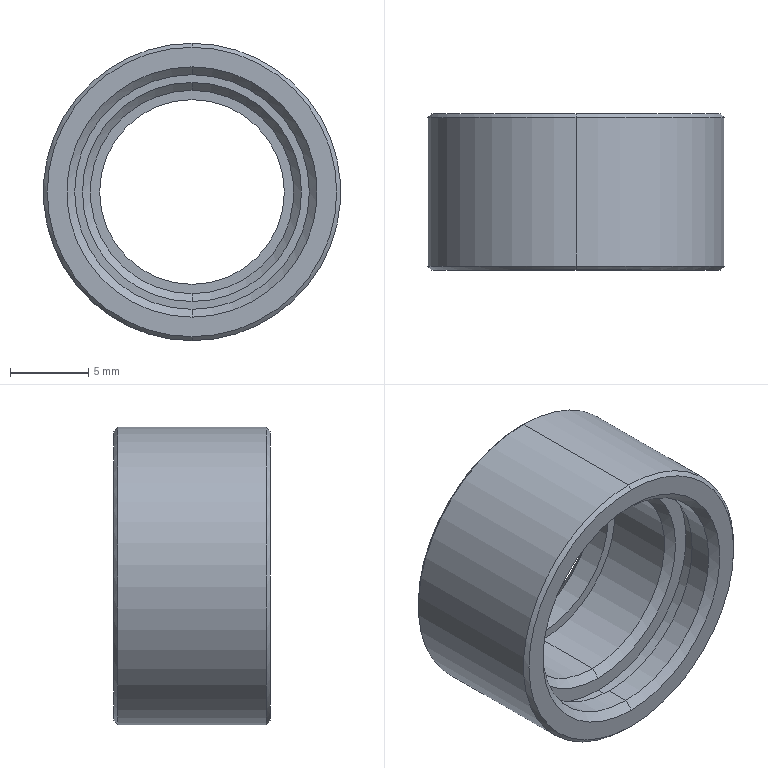Part | NX | features BREP 1 | 1 solid | 25 faces | box 19 x 10 x 19 mm | volume 1381 mm3 | cone 10 | cylinder 10 | plane 5 | commonest cylinder face diameters 11.8 x2 13 x2 15 x2 15.9 x2 19 x2
STEP:
#1=CARTESIAN_POINT('',(0.,0.25,-9.5));
#2=VERTEX_POINT('',#1);
#3=CARTESIAN_POINT('',(0.,0.,-9.25));
#4=VERTEX_POINT('',#3);
#5=CARTESIAN_POINT('',(0.,0.,-9.25));
#6=DIRECTION('',(0.,0.7071,-0.7071));
#7=VECTOR('',#6,1000.);
#8=LINE('',#5,#7);
#9=EDGE_CURVE('',#2,#4,#8,.F.);
#10=ORIENTED_EDGE('',*,*,#9,.T.);
#11=CARTESIAN_POINT('',(0.,0.,9.25));
#12=VERTEX_POINT('',#11);
#13=CARTESIAN_POINT('',(0.,0.,0.));
#14=DIRECTION('',(0.,-1.,0.));
#15=DIRECTION('',(0.,0.,1.));
#16=AXIS2_PLACEMENT_3D('',#13,#14,#15);
#17=CIRCLE('',#16,9.25);
#18=EDGE_CURVE('',#12,#4,#17,.T.);
#19=ORIENTED_EDGE('',*,*,#18,.F.);
#20=CARTESIAN_POINT('',(0.,0.25,9.5));
#21=VERTEX_POINT('',#20);
#22=CARTESIAN_POINT('',(0.,0.,9.25));
#23=DIRECTION('',(0.,0.7071,0.7071));
#24=VECTOR('',#23,1000.);
#25=LINE('',#22,#24);
#26=EDGE_CURVE('',#21,#12,#25,.F.);
#27=ORIENTED_EDGE('',*,*,#26,.F.);
#28=CARTESIAN_POINT('',(0.,0.25,0.));
#29=DIRECTION('',(0.,1.,0.));
#30=DIRECTION('',(0.,0.,1.));
#31=AXIS2_PLACEMENT_3D('',#28,#29,#30);
#32=CIRCLE('',#31,9.5);
#33=EDGE_CURVE('',#2,#21,#32,.T.);
#34=ORIENTED_EDGE('',*,*,#33,.F.);
#35=EDGE_LOOP('',(#10,#19,#27,#34));
#36=FACE_BOUND('',#35,.T.);
#37=CARTESIAN_POINT('',(0.,0.,0.));
#38=DIRECTION('',(0.,1.,0.));
#39=DIRECTION('',(0.,0.,1.));
#40=AXIS2_PLACEMENT_3D('',#37,#38,#39);
#41=CONICAL_SURFACE('',#40,9.25,0.7854);
#42=ADVANCED_FACE('',(#36),#41,.T.);
#43=CARTESIAN_POINT('',(0.,10.,9.25));
#44=VERTEX_POINT('',#43);
#45=CARTESIAN_POINT('',(0.,9.75,9.5));
#46=VERTEX_POINT('',#45);
#47=CARTESIAN_POINT('',(0.,9.75,9.5));
#48=DIRECTION('',(0.,-0.7071,0.7071));
#49=VECTOR('',#48,1000.);
#50=LINE('',#47,#49);
#51=EDGE_CURVE('',#44,#46,#50,.T.);
#52=ORIENTED_EDGE('',*,*,#51,.F.);
#53=CARTESIAN_POINT('',(0.,10.,-9.25));
#54=VERTEX_POINT('',#53);
#55=CARTESIAN_POINT('',(0.,10.,0.));
#56=DIRECTION('',(0.,1.,0.));
#57=DIRECTION('',(0.,0.,-1.));
#58=AXIS2_PLACEMENT_3D('',#55,#56,#57);
#59=CIRCLE('',#58,9.25);
#60=EDGE_CURVE('',#54,#44,#59,.T.);
#61=ORIENTED_EDGE('',*,*,#60,.F.);
#62=CARTESIAN_POINT('',(0.,9.75,-9.5));
#63=VERTEX_POINT('',#62);
#64=CARTESIAN_POINT('',(0.,9.75,-9.5));
#65=DIRECTION('',(0.,-0.7071,-0.7071));
#66=VECTOR('',#65,1000.);
#67=LINE('',#64,#66);
#68=EDGE_CURVE('',#54,#63,#67,.T.);
#69=ORIENTED_EDGE('',*,*,#68,.T.);
#70=CARTESIAN_POINT('',(0.,9.75,0.));
#71=DIRECTION('',(0.,-1.,0.));
#72=DIRECTION('',(0.,0.,-1.));
#73=AXIS2_PLACEMENT_3D('',#70,#71,#72);
#74=CIRCLE('',#73,9.5);
#75=EDGE_CURVE('',#46,#63,#74,.T.);
#76=ORIENTED_EDGE('',*,*,#75,.F.);
#77=EDGE_LOOP('',(#52,#61,#69,#76));
#78=FACE_BOUND('',#77,.T.);
#79=CARTESIAN_POINT('',(0.,9.75,0.));
#80=DIRECTION('',(0.,-1.,0.));
#81=DIRECTION('',(0.,0.,-1.));
#82=AXIS2_PLACEMENT_3D('',#79,#80,#81);
#83=CONICAL_SURFACE('',#82,9.5,0.7854);
#84=ADVANCED_FACE('',(#78),#83,.T.);
#85=CARTESIAN_POINT('',(0.,10.,-6.4));
#86=VERTEX_POINT('',#85);
#87=CARTESIAN_POINT('',(0.,9.5,-5.9));
#88=VERTEX_POINT('',#87);
#89=CARTESIAN_POINT('',(0.,10.,-6.4));
#90=DIRECTION('',(0.,0.7071,-0.7071));
#91=VECTOR('',#90,1000.);
#92=LINE('',#89,#91);
#93=EDGE_CURVE('',#86,#88,#92,.F.);
#94=ORIENTED_EDGE('',*,*,#93,.T.);
#95=CARTESIAN_POINT('',(0.,9.5,5.9));
#96=VERTEX_POINT('',#95);
#97=CARTESIAN_POINT('',(0.,9.5,0.));
#98=DIRECTION('',(0.,1.,0.));
#99=DIRECTION('',(0.,0.,-1.));
#100=AXIS2_PLACEMENT_3D('',#97,#98,#99);
#101=CIRCLE('',#100,5.9);
#102=EDGE_CURVE('',#96,#88,#101,.T.);
#103=ORIENTED_EDGE('',*,*,#102,.F.);
#104=CARTESIAN_POINT('',(0.,10.,6.4));
#105=VERTEX_POINT('',#104);
#106=CARTESIAN_POINT('',(0.,10.,6.4));
#107=DIRECTION('',(0.,0.7071,0.7071));
#108=VECTOR('',#107,1000.);
#109=LINE('',#106,#108);
#110=EDGE_CURVE('',#105,#96,#109,.F.);
#111=ORIENTED_EDGE('',*,*,#110,.F.);
#112=CARTESIAN_POINT('',(0.,10.,0.));
#113=DIRECTION('',(0.,-1.,0.));
#114=DIRECTION('',(0.,0.,-1.));
#115=AXIS2_PLACEMENT_3D('',#112,#113,#114);
#116=CIRCLE('',#115,6.4);
#117=EDGE_CURVE('',#86,#105,#116,.T.);
#118=ORIENTED_EDGE('',*,*,#117,.F.);
#119=EDGE_LOOP('',(#94,#103,#111,#118));
#120=FACE_BOUND('',#119,.T.);
#121=CARTESIAN_POINT('',(0.,10.,0.));
#122=DIRECTION('',(0.,1.,0.));
#123=DIRECTION('',(0.,0.,1.));
#124=AXIS2_PLACEMENT_3D('',#121,#122,#123);
#125=CONICAL_SURFACE('',#124,6.4,0.7854);
#126=ADVANCED_FACE('',(#120),#125,.F.);
#127=CARTESIAN_POINT('',(0.,3.5,6.5));
#128=VERTEX_POINT('',#127);
#129=CARTESIAN_POINT('',(0.,3.,7.));
#130=VERTEX_POINT('',#129);
#131=CARTESIAN_POINT('',(0.,3.5,6.5));
#132=DIRECTION('',(0.,-0.7071,0.7071));
#133=VECTOR('',#132,1000.);
#134=LINE('',#131,#133);
#135=EDGE_CURVE('',#128,#130,#134,.T.);
#136=ORIENTED_EDGE('',*,*,#135,.F.);
#137=CARTESIAN_POINT('',(0.,3.5,-6.5));
#138=VERTEX_POINT('',#137);
#139=CARTESIAN_POINT('',(0.,3.5,0.));
#140=DIRECTION('',(0.,-1.,0.));
#141=DIRECTION('',(0.,0.,1.));
#142=AXIS2_PLACEMENT_3D('',#139,#140,#141);
#143=CIRCLE('',#142,6.5);
#144=EDGE_CURVE('',#138,#128,#143,.T.);
#145=ORIENTED_EDGE('',*,*,#144,.F.);
#146=CARTESIAN_POINT('',(0.,3.,-7.));
#147=VERTEX_POINT('',#146);
#148=CARTESIAN_POINT('',(0.,3.5,-6.5));
#149=DIRECTION('',(0.,-0.7071,-0.7071));
#150=VECTOR('',#149,1000.);
#151=LINE('',#148,#150);
#152=EDGE_CURVE('',#138,#147,#151,.T.);
#153=ORIENTED_EDGE('',*,*,#152,.T.);
#154=CARTESIAN_POINT('',(0.,3.,0.));
#155=DIRECTION('',(0.,1.,0.));
#156=DIRECTION('',(0.,0.,1.));
#157=AXIS2_PLACEMENT_3D('',#154,#155,#156);
#158=CIRCLE('',#157,7.);
#159=EDGE_CURVE('',#130,#147,#158,.T.);
#160=ORIENTED_EDGE('',*,*,#159,.F.);
#161=EDGE_LOOP('',(#136,#145,#153,#160));
#162=FACE_BOUND('',#161,.T.);
#163=CARTESIAN_POINT('',(0.,3.5,0.));
#164=DIRECTION('',(0.,-1.,0.));
#165=DIRECTION('',(0.,0.,-1.));
#166=AXIS2_PLACEMENT_3D('',#163,#164,#165);
#167=CONICAL_SURFACE('',#166,6.5,0.7854);
#168=ADVANCED_FACE('',(#162),#167,.F.);
#169=CARTESIAN_POINT('',(0.,0.5,7.5));
#170=VERTEX_POINT('',#169);
#171=CARTESIAN_POINT('',(0.,0.,8.));
#172=VERTEX_POINT('',#171);
#173=CARTESIAN_POINT('',(0.,0.5,7.5));
#174=DIRECTION('',(0.,-0.7071,0.7071));
#175=VECTOR('',#174,1000.);
#176=LINE('',#173,#175);
#177=EDGE_CURVE('',#170,#172,#176,.T.);
#178=ORIENTED_EDGE('',*,*,#177,.F.);
#179=CARTESIAN_POINT('',(0.,0.5,-7.5));
#180=VERTEX_POINT('',#179);
#181=CARTESIAN_POINT('',(0.,0.5,0.));
#182=DIRECTION('',(0.,-1.,0.));
#183=DIRECTION('',(0.,0.,1.));
#184=AXIS2_PLACEMENT_3D('',#181,#182,#183);
#185=CIRCLE('',#184,7.5);
#186=EDGE_CURVE('',#180,#170,#185,.T.);
#187=ORIENTED_EDGE('',*,*,#186,.F.);
#188=CARTESIAN_POINT('',(0.,0.,-8.));
#189=VERTEX_POINT('',#188);
#190=CARTESIAN_POINT('',(0.,0.5,-7.5));
#191=DIRECTION('',(0.,-0.7071,-0.7071));
#192=VECTOR('',#191,1000.);
#193=LINE('',#190,#192);
#194=EDGE_CURVE('',#180,#189,#193,.T.);
#195=ORIENTED_EDGE('',*,*,#194,.T.);
#196=CARTESIAN_POINT('',(0.,0.,0.));
#197=DIRECTION('',(0.,1.,0.));
#198=DIRECTION('',(0.,0.,1.));
#199=AXIS2_PLACEMENT_3D('',#196,#197,#198);
#200=CIRCLE('',#199,8.);
#201=EDGE_CURVE('',#172,#189,#200,.T.);
#202=ORIENTED_EDGE('',*,*,#201,.F.);
#203=EDGE_LOOP('',(#178,#187,#195,#202));
#204=FACE_BOUND('',#203,.T.);
#205=CARTESIAN_POINT('',(0.,0.5,0.));
#206=DIRECTION('',(0.,-1.,0.));
#207=DIRECTION('',(0.,0.,-1.));
#208=AXIS2_PLACEMENT_3D('',#205,#206,#207);
#209=CONICAL_SURFACE('',#208,7.5,0.7854);
#210=ADVANCED_FACE('',(#204),#209,.F.);
#211=CARTESIAN_POINT('',(0.,2.,7.5));
#212=VERTEX_POINT('',#211);
#213=CARTESIAN_POINT('',(0.,0.,7.5));
#214=DIRECTION('',(0.,-1.,0.));
#215=VECTOR('',#214,1000.);
#216=LINE('',#213,#215);
#217=EDGE_CURVE('',#212,#170,#216,.T.);
#218=ORIENTED_EDGE('',*,*,#217,.F.);
#219=CARTESIAN_POINT('',(0.,2.,-7.5));
#220=VERTEX_POINT('',#219);
#221=CARTESIAN_POINT('',(0.,2.,0.));
#222=DIRECTION('',(0.,-1.,0.));
#223=DIRECTION('',(0.,0.,-1.));
#224=AXIS2_PLACEMENT_3D('',#221,#222,#223);
#225=CIRCLE('',#224,7.5);
#226=EDGE_CURVE('',#220,#212,#225,.T.);
#227=ORIENTED_EDGE('',*,*,#226,.F.);
#228=CARTESIAN_POINT('',(0.,0.,-7.5));
#229=DIRECTION('',(0.,-1.,0.));
#230=VECTOR('',#229,1000.);
#231=LINE('',#228,#230);
#232=EDGE_CURVE('',#220,#180,#231,.T.);
#233=ORIENTED_EDGE('',*,*,#232,.T.);
#234=ORIENTED_EDGE('',*,*,#186,.T.);
#235=EDGE_LOOP('',(#218,#227,#233,#234));
#236=FACE_BOUND('',#235,.T.);
#237=CARTESIAN_POINT('',(0.,0.,0.));
#238=DIRECTION('',(0.,-1.,0.));
#239=DIRECTION('',(0.,0.,-1.));
#240=AXIS2_PLACEMENT_3D('',#237,#238,#239);
#241=CYLINDRICAL_SURFACE('',#240,7.5);
#242=ADVANCED_FACE('',(#236),#241,.F.);
#243=ORIENTED_EDGE('',*,*,#226,.T.);
#244=CARTESIAN_POINT('',(0.,2.,0.));
#245=DIRECTION('',(0.,-1.,0.));
#246=DIRECTION('',(0.,0.,-1.));
#247=AXIS2_PLACEMENT_3D('',#244,#245,#246);
#248=CIRCLE('',#247,7.5);
#249=EDGE_CURVE('',#212,#220,#248,.T.);
#250=ORIENTED_EDGE('',*,*,#249,.T.);
#251=EDGE_LOOP('',(#243,#250));
#252=FACE_BOUND('',#251,.T.);
#253=CARTESIAN_POINT('',(0.,2.,-7.95));
#254=VERTEX_POINT('',#253);
#255=CARTESIAN_POINT('',(0.,2.,7.95));
#256=VERTEX_POINT('',#255);
#257=CARTESIAN_POINT('',(0.,2.,0.));
#258=DIRECTION('',(0.,-1.,0.));
#259=DIRECTION('',(0.,0.,-1.));
#260=AXIS2_PLACEMENT_3D('',#257,#258,#259);
#261=CIRCLE('',#260,7.95);
#262=EDGE_CURVE('',#254,#256,#261,.T.);
#263=ORIENTED_EDGE('',*,*,#262,.F.);
#264=CARTESIAN_POINT('',(0.,2.,0.));
#265=DIRECTION('',(0.,-1.,0.));
#266=DIRECTION('',(0.,0.,-1.));
#267=AXIS2_PLACEMENT_3D('',#264,#265,#266);
#268=CIRCLE('',#267,7.95);
#269=EDGE_CURVE('',#256,#254,#268,.T.);
#270=ORIENTED_EDGE('',*,*,#269,.F.);
#271=EDGE_LOOP('',(#263,#270));
#272=FACE_BOUND('',#271,.T.);
#273=CARTESIAN_POINT('',(-7.95,2.,0.));
#274=DIRECTION('',(0.,-1.,0.));
#275=DIRECTION('',(0.,0.,-1.));
#276=AXIS2_PLACEMENT_3D('',#273,#274,#275);
#277=PLANE('',#276);
#278=ADVANCED_FACE('',(#252,#272),#277,.F.);
#279=CARTESIAN_POINT('',(0.,3.,7.95));
#280=VERTEX_POINT('',#279);
#281=CARTESIAN_POINT('',(0.,0.,7.95));
#282=DIRECTION('',(0.,-1.,0.));
#283=VECTOR('',#282,1000.);
#284=LINE('',#281,#283);
#285=EDGE_CURVE('',#280,#256,#284,.T.);
#286=ORIENTED_EDGE('',*,*,#285,.F.);
#287=CARTESIAN_POINT('',(0.,3.,-7.95));
#288=VERTEX_POINT('',#287);
#289=CARTESIAN_POINT('',(0.,3.,0.));
#290=DIRECTION('',(0.,-1.,0.));
#291=DIRECTION('',(0.,0.,-1.));
#292=AXIS2_PLACEMENT_3D('',#289,#290,#291);
#293=CIRCLE('',#292,7.95);
#294=EDGE_CURVE('',#288,#280,#293,.T.);
#295=ORIENTED_EDGE('',*,*,#294,.F.);
#296=CARTESIAN_POINT('',(0.,0.,-7.95));
#297=DIRECTION('',(0.,-1.,0.));
#298=VECTOR('',#297,1000.);
#299=LINE('',#296,#298);
#300=EDGE_CURVE('',#288,#254,#299,.T.);
#301=ORIENTED_EDGE('',*,*,#300,.T.);
#302=ORIENTED_EDGE('',*,*,#262,.T.);
#303=EDGE_LOOP('',(#286,#295,#301,#302));
#304=FACE_BOUND('',#303,.T.);
#305=CARTESIAN_POINT('',(0.,0.,0.));
#306=DIRECTION('',(0.,-1.,0.));
#307=DIRECTION('',(0.,0.,-1.));
#308=AXIS2_PLACEMENT_3D('',#305,#306,#307);
#309=CYLINDRICAL_SURFACE('',#308,7.95);
#310=ADVANCED_FACE('',(#304),#309,.F.);
#311=ORIENTED_EDGE('',*,*,#294,.T.);
#312=CARTESIAN_POINT('',(0.,3.,0.));
#313=DIRECTION('',(0.,-1.,0.));
#314=DIRECTION('',(0.,0.,-1.));
#315=AXIS2_PLACEMENT_3D('',#312,#313,#314);
#316=CIRCLE('',#315,7.95);
#317=EDGE_CURVE('',#280,#288,#316,.T.);
#318=ORIENTED_EDGE('',*,*,#317,.T.);
#319=EDGE_LOOP('',(#311,#318));
#320=FACE_BOUND('',#319,.T.);
#321=CARTESIAN_POINT('',(0.,3.,0.));
#322=DIRECTION('',(0.,1.,0.));
#323=DIRECTION('',(0.,0.,1.));
#324=AXIS2_PLACEMENT_3D('',#321,#322,#323);
#325=CIRCLE('',#324,7.);
#326=EDGE_CURVE('',#147,#130,#325,.T.);
#327=ORIENTED_EDGE('',*,*,#326,.T.);
#328=ORIENTED_EDGE('',*,*,#159,.T.);
#329=EDGE_LOOP('',(#327,#328));
#330=FACE_BOUND('',#329,.T.);
#331=CARTESIAN_POINT('',(-6.5,3.,0.));
#332=DIRECTION('',(0.,1.,0.));
#333=DIRECTION('',(0.,0.,1.));
#334=AXIS2_PLACEMENT_3D('',#331,#332,#333);
#335=PLANE('',#334);
#336=ADVANCED_FACE('',(#320,#330),#335,.F.);
#337=CARTESIAN_POINT('',(0.,8.,6.5));
#338=VERTEX_POINT('',#337);
#339=CARTESIAN_POINT('',(0.,0.,6.5));
#340=DIRECTION('',(0.,-1.,0.));
#341=VECTOR('',#340,1000.);
#342=LINE('',#339,#341);
#343=EDGE_CURVE('',#338,#128,#342,.T.);
#344=ORIENTED_EDGE('',*,*,#343,.F.);
#345=CARTESIAN_POINT('',(0.,8.,-6.5));
#346=VERTEX_POINT('',#345);
#347=CARTESIAN_POINT('',(0.,8.,0.));
#348=DIRECTION('',(0.,-1.,0.));
#349=DIRECTION('',(0.,0.,-1.));
#350=AXIS2_PLACEMENT_3D('',#347,#348,#349);
#351=CIRCLE('',#350,6.5);
#352=EDGE_CURVE('',#346,#338,#351,.T.);
#353=ORIENTED_EDGE('',*,*,#352,.F.);
#354=CARTESIAN_POINT('',(0.,0.,-6.5));
#355=DIRECTION('',(0.,-1.,0.));
#356=VECTOR('',#355,1000.);
#357=LINE('',#354,#356);
#358=EDGE_CURVE('',#346,#138,#357,.T.);
#359=ORIENTED_EDGE('',*,*,#358,.T.);
#360=ORIENTED_EDGE('',*,*,#144,.T.);
#361=EDGE_LOOP('',(#344,#353,#359,#360));
#362=FACE_BOUND('',#361,.T.);
#363=CARTESIAN_POINT('',(0.,0.,0.));
#364=DIRECTION('',(0.,-1.,0.));
#365=DIRECTION('',(0.,0.,-1.));
#366=AXIS2_PLACEMENT_3D('',#363,#364,#365);
#367=CYLINDRICAL_SURFACE('',#366,6.5);
#368=ADVANCED_FACE('',(#362),#367,.F.);
#369=ORIENTED_EDGE('',*,*,#352,.T.);
#370=CARTESIAN_POINT('',(0.,8.,0.));
#371=DIRECTION('',(0.,-1.,0.));
#372=DIRECTION('',(0.,0.,-1.));
#373=AXIS2_PLACEMENT_3D('',#370,#371,#372);
#374=CIRCLE('',#373,6.5);
#375=EDGE_CURVE('',#338,#346,#374,.T.);
#376=ORIENTED_EDGE('',*,*,#375,.T.);
#377=EDGE_LOOP('',(#369,#376));
#378=FACE_BOUND('',#377,.T.);
#379=CARTESIAN_POINT('',(0.,8.,-5.9));
#380=VERTEX_POINT('',#379);
#381=CARTESIAN_POINT('',(0.,8.,5.9));
#382=VERTEX_POINT('',#381);
#383=CARTESIAN_POINT('',(0.,8.,0.));
#384=DIRECTION('',(0.,-1.,0.));
#385=DIRECTION('',(0.,0.,-1.));
#386=AXIS2_PLACEMENT_3D('',#383,#384,#385);
#387=CIRCLE('',#386,5.9);
#388=EDGE_CURVE('',#380,#382,#387,.T.);
#389=ORIENTED_EDGE('',*,*,#388,.F.);
#390=CARTESIAN_POINT('',(0.,8.,0.));
#391=DIRECTION('',(0.,-1.,0.));
#392=DIRECTION('',(0.,0.,-1.));
#393=AXIS2_PLACEMENT_3D('',#390,#391,#392);
#394=CIRCLE('',#393,5.9);
#395=EDGE_CURVE('',#382,#380,#394,.T.);
#396=ORIENTED_EDGE('',*,*,#395,.F.);
#397=EDGE_LOOP('',(#389,#396));
#398=FACE_BOUND('',#397,.T.);
#399=CARTESIAN_POINT('',(-5.9,8.,0.));
#400=DIRECTION('',(0.,1.,0.));
#401=DIRECTION('',(0.,0.,1.));
#402=AXIS2_PLACEMENT_3D('',#399,#400,#401);
#403=PLANE('',#402);
#404=ADVANCED_FACE('',(#378,#398),#403,.F.);
#405=CARTESIAN_POINT('',(0.,0.,5.9));
#406=DIRECTION('',(0.,-1.,0.));
#407=VECTOR('',#406,1000.);
#408=LINE('',#405,#407);
#409=EDGE_CURVE('',#96,#382,#408,.T.);
#410=ORIENTED_EDGE('',*,*,#409,.F.);
#411=ORIENTED_EDGE('',*,*,#102,.T.);
#412=CARTESIAN_POINT('',(0.,0.,-5.9));
#413=DIRECTION('',(0.,-1.,0.));
#414=VECTOR('',#413,1000.);
#415=LINE('',#412,#414);
#416=EDGE_CURVE('',#88,#380,#415,.T.);
#417=ORIENTED_EDGE('',*,*,#416,.T.);
#418=ORIENTED_EDGE('',*,*,#388,.T.);
#419=EDGE_LOOP('',(#410,#411,#417,#418));
#420=FACE_BOUND('',#419,.T.);
#421=CARTESIAN_POINT('',(0.,0.,0.));
#422=DIRECTION('',(0.,-1.,0.));
#423=DIRECTION('',(0.,0.,-1.));
#424=AXIS2_PLACEMENT_3D('',#421,#422,#423);
#425=CYLINDRICAL_SURFACE('',#424,5.9);
#426=ADVANCED_FACE('',(#420),#425,.F.);
#427=CARTESIAN_POINT('',(0.,10.,0.));
#428=DIRECTION('',(0.,-1.,0.));
#429=DIRECTION('',(0.,0.,-1.));
#430=AXIS2_PLACEMENT_3D('',#427,#428,#429);
#431=CIRCLE('',#430,6.4);
#432=EDGE_CURVE('',#105,#86,#431,.T.);
#433=ORIENTED_EDGE('',*,*,#432,.T.);
#434=ORIENTED_EDGE('',*,*,#117,.T.);
#435=EDGE_LOOP('',(#433,#434));
#436=FACE_BOUND('',#435,.T.);
#437=ORIENTED_EDGE('',*,*,#60,.T.);
#438=CARTESIAN_POINT('',(0.,10.,0.));
#439=DIRECTION('',(0.,1.,0.));
#440=DIRECTION('',(0.,0.,-1.));
#441=AXIS2_PLACEMENT_3D('',#438,#439,#440);
#442=CIRCLE('',#441,9.25);
#443=EDGE_CURVE('',#44,#54,#442,.T.);
#444=ORIENTED_EDGE('',*,*,#443,.T.);
#445=EDGE_LOOP('',(#437,#444));
#446=FACE_BOUND('',#445,.T.);
#447=CARTESIAN_POINT('',(-5.9,10.,0.));
#448=DIRECTION('',(0.,-1.,0.));
#449=DIRECTION('',(0.,0.,-1.));
#450=AXIS2_PLACEMENT_3D('',#447,#448,#449);
#451=PLANE('',#450);
#452=ADVANCED_FACE('',(#436,#446),#451,.F.);
#453=CARTESIAN_POINT('',(0.,0.,9.5));
#454=DIRECTION('',(0.,-1.,0.));
#455=VECTOR('',#454,1000.);
#456=LINE('',#453,#455);
#457=EDGE_CURVE('',#46,#21,#456,.T.);
#458=ORIENTED_EDGE('',*,*,#457,.F.);
#459=ORIENTED_EDGE('',*,*,#75,.T.);
#460=CARTESIAN_POINT('',(0.,0.,-9.5));
#461=DIRECTION('',(0.,-1.,0.));
#462=VECTOR('',#461,1000.);
#463=LINE('',#460,#462);
#464=EDGE_CURVE('',#63,#2,#463,.T.);
#465=ORIENTED_EDGE('',*,*,#464,.T.);
#466=ORIENTED_EDGE('',*,*,#33,.T.);
#467=EDGE_LOOP('',(#458,#459,#465,#466));
#468=FACE_BOUND('',#467,.T.);
#469=CARTESIAN_POINT('',(0.,0.,0.));
#470=DIRECTION('',(0.,-1.,0.));
#471=DIRECTION('',(0.,0.,-1.));
#472=AXIS2_PLACEMENT_3D('',#469,#470,#471);
#473=CYLINDRICAL_SURFACE('',#472,9.5);
#474=ADVANCED_FACE('',(#468),#473,.T.);
#475=CARTESIAN_POINT('',(0.,0.,0.));
#476=DIRECTION('',(0.,1.,0.));
#477=DIRECTION('',(0.,0.,1.));
#478=AXIS2_PLACEMENT_3D('',#475,#476,#477);
#479=CIRCLE('',#478,8.);
#480=EDGE_CURVE('',#189,#172,#479,.T.);
#481=ORIENTED_EDGE('',*,*,#480,.T.);
#482=ORIENTED_EDGE('',*,*,#201,.T.);
#483=EDGE_LOOP('',(#481,#482));
#484=FACE_BOUND('',#483,.T.);
#485=ORIENTED_EDGE('',*,*,#18,.T.);
#486=CARTESIAN_POINT('',(0.,0.,0.));
#487=DIRECTION('',(0.,-1.,0.));
#488=DIRECTION('',(0.,0.,1.));
#489=AXIS2_PLACEMENT_3D('',#486,#487,#488);
#490=CIRCLE('',#489,9.25);
#491=EDGE_CURVE('',#4,#12,#490,.T.);
#492=ORIENTED_EDGE('',*,*,#491,.T.);
#493=EDGE_LOOP('',(#485,#492));
#494=FACE_BOUND('',#493,.T.);
#495=CARTESIAN_POINT('',(-9.5,0.,0.));
#496=DIRECTION('',(0.,1.,0.));
#497=DIRECTION('',(0.,0.,1.));
#498=AXIS2_PLACEMENT_3D('',#495,#496,#497);
#499=PLANE('',#498);
#500=ADVANCED_FACE('',(#484,#494),#499,.F.);
#501=CARTESIAN_POINT('',(0.,9.75,0.));
#502=DIRECTION('',(0.,-1.,0.));
#503=DIRECTION('',(0.,0.,-1.));
#504=AXIS2_PLACEMENT_3D('',#501,#502,#503);
#505=CIRCLE('',#504,9.5);
#506=EDGE_CURVE('',#63,#46,#505,.T.);
#507=ORIENTED_EDGE('',*,*,#506,.T.);
#508=ORIENTED_EDGE('',*,*,#457,.T.);
#509=CARTESIAN_POINT('',(0.,0.25,0.));
#510=DIRECTION('',(0.,1.,0.));
#511=DIRECTION('',(0.,0.,1.));
#512=AXIS2_PLACEMENT_3D('',#509,#510,#511);
#513=CIRCLE('',#512,9.5);
#514=EDGE_CURVE('',#21,#2,#513,.T.);
#515=ORIENTED_EDGE('',*,*,#514,.T.);
#516=ORIENTED_EDGE('',*,*,#464,.F.);
#517=EDGE_LOOP('',(#507,#508,#515,#516));
#518=FACE_BOUND('',#517,.T.);
#519=CARTESIAN_POINT('',(0.,0.,0.));
#520=DIRECTION('',(0.,-1.,0.));
#521=DIRECTION('',(0.,0.,-1.));
#522=AXIS2_PLACEMENT_3D('',#519,#520,#521);
#523=CYLINDRICAL_SURFACE('',#522,9.5);
#524=ADVANCED_FACE('',(#518),#523,.T.);
#525=CARTESIAN_POINT('',(0.,9.5,0.));
#526=DIRECTION('',(0.,1.,0.));
#527=DIRECTION('',(0.,0.,-1.));
#528=AXIS2_PLACEMENT_3D('',#525,#526,#527);
#529=CIRCLE('',#528,5.9);
#530=EDGE_CURVE('',#88,#96,#529,.T.);
#531=ORIENTED_EDGE('',*,*,#530,.T.);
#532=ORIENTED_EDGE('',*,*,#409,.T.);
#533=ORIENTED_EDGE('',*,*,#395,.T.);
#534=ORIENTED_EDGE('',*,*,#416,.F.);
#535=EDGE_LOOP('',(#531,#532,#533,#534));
#536=FACE_BOUND('',#535,.T.);
#537=CARTESIAN_POINT('',(0.,0.,0.));
#538=DIRECTION('',(0.,-1.,0.));
#539=DIRECTION('',(0.,0.,-1.));
#540=AXIS2_PLACEMENT_3D('',#537,#538,#539);
#541=CYLINDRICAL_SURFACE('',#540,5.9);
#542=ADVANCED_FACE('',(#536),#541,.F.);
#543=ORIENTED_EDGE('',*,*,#375,.F.);
#544=ORIENTED_EDGE('',*,*,#343,.T.);
#545=CARTESIAN_POINT('',(0.,3.5,0.));
#546=DIRECTION('',(0.,-1.,0.));
#547=DIRECTION('',(0.,0.,1.));
#548=AXIS2_PLACEMENT_3D('',#545,#546,#547);
#549=CIRCLE('',#548,6.5);
#550=EDGE_CURVE('',#128,#138,#549,.T.);
#551=ORIENTED_EDGE('',*,*,#550,.T.);
#552=ORIENTED_EDGE('',*,*,#358,.F.);
#553=EDGE_LOOP('',(#543,#544,#551,#552));
#554=FACE_BOUND('',#553,.T.);
#555=CARTESIAN_POINT('',(0.,0.,0.));
#556=DIRECTION('',(0.,-1.,0.));
#557=DIRECTION('',(0.,0.,-1.));
#558=AXIS2_PLACEMENT_3D('',#555,#556,#557);
#559=CYLINDRICAL_SURFACE('',#558,6.5);
#560=ADVANCED_FACE('',(#554),#559,.F.);
#561=ORIENTED_EDGE('',*,*,#317,.F.);
#562=ORIENTED_EDGE('',*,*,#285,.T.);
#563=ORIENTED_EDGE('',*,*,#269,.T.);
#564=ORIENTED_EDGE('',*,*,#300,.F.);
#565=EDGE_LOOP('',(#561,#562,#563,#564));
#566=FACE_BOUND('',#565,.T.);
#567=CARTESIAN_POINT('',(0.,0.,0.));
#568=DIRECTION('',(0.,-1.,0.));
#569=DIRECTION('',(0.,0.,-1.));
#570=AXIS2_PLACEMENT_3D('',#567,#568,#569);
#571=CYLINDRICAL_SURFACE('',#570,7.95);
#572=ADVANCED_FACE('',(#566),#571,.F.);
#573=ORIENTED_EDGE('',*,*,#249,.F.);
#574=ORIENTED_EDGE('',*,*,#217,.T.);
#575=CARTESIAN_POINT('',(0.,0.5,0.));
#576=DIRECTION('',(0.,-1.,0.));
#577=DIRECTION('',(0.,0.,1.));
#578=AXIS2_PLACEMENT_3D('',#575,#576,#577);
#579=CIRCLE('',#578,7.5);
#580=EDGE_CURVE('',#170,#180,#579,.T.);
#581=ORIENTED_EDGE('',*,*,#580,.T.);
#582=ORIENTED_EDGE('',*,*,#232,.F.);
#583=EDGE_LOOP('',(#573,#574,#581,#582));
#584=FACE_BOUND('',#583,.T.);
#585=CARTESIAN_POINT('',(0.,0.,0.));
#586=DIRECTION('',(0.,-1.,0.));
#587=DIRECTION('',(0.,0.,-1.));
#588=AXIS2_PLACEMENT_3D('',#585,#586,#587);
#589=CYLINDRICAL_SURFACE('',#588,7.5);
#590=ADVANCED_FACE('',(#584),#589,.F.);
#591=ORIENTED_EDGE('',*,*,#580,.F.);
#592=ORIENTED_EDGE('',*,*,#177,.T.);
#593=ORIENTED_EDGE('',*,*,#480,.F.);
#594=ORIENTED_EDGE('',*,*,#194,.F.);
#595=EDGE_LOOP('',(#591,#592,#593,#594));
#596=FACE_BOUND('',#595,.T.);
#597=CARTESIAN_POINT('',(0.,0.5,0.));
#598=DIRECTION('',(0.,-1.,0.));
#599=DIRECTION('',(0.,0.,-1.));
#600=AXIS2_PLACEMENT_3D('',#597,#598,#599);
#601=CONICAL_SURFACE('',#600,7.5,0.7854);
#602=ADVANCED_FACE('',(#596),#601,.F.);
#603=ORIENTED_EDGE('',*,*,#550,.F.);
#604=ORIENTED_EDGE('',*,*,#135,.T.);
#605=ORIENTED_EDGE('',*,*,#326,.F.);
#606=ORIENTED_EDGE('',*,*,#152,.F.);
#607=EDGE_LOOP('',(#603,#604,#605,#606));
#608=FACE_BOUND('',#607,.T.);
#609=CARTESIAN_POINT('',(0.,3.5,0.));
#610=DIRECTION('',(0.,-1.,0.));
#611=DIRECTION('',(0.,0.,-1.));
#612=AXIS2_PLACEMENT_3D('',#609,#610,#611);
#613=CONICAL_SURFACE('',#612,6.5,0.7854);
#614=ADVANCED_FACE('',(#608),#613,.F.);
#615=ORIENTED_EDGE('',*,*,#530,.F.);
#616=ORIENTED_EDGE('',*,*,#93,.F.);
#617=ORIENTED_EDGE('',*,*,#432,.F.);
#618=ORIENTED_EDGE('',*,*,#110,.T.);
#619=EDGE_LOOP('',(#615,#616,#617,#618));
#620=FACE_BOUND('',#619,.T.);
#621=CARTESIAN_POINT('',(0.,10.,0.));
#622=DIRECTION('',(0.,1.,0.));
#623=DIRECTION('',(0.,0.,1.));
#624=AXIS2_PLACEMENT_3D('',#621,#622,#623);
#625=CONICAL_SURFACE('',#624,6.4,0.7854);
#626=ADVANCED_FACE('',(#620),#625,.F.);
#627=ORIENTED_EDGE('',*,*,#443,.F.);
#628=ORIENTED_EDGE('',*,*,#51,.T.);
#629=ORIENTED_EDGE('',*,*,#506,.F.);
#630=ORIENTED_EDGE('',*,*,#68,.F.);
#631=EDGE_LOOP('',(#627,#628,#629,#630));
#632=FACE_BOUND('',#631,.T.);
#633=CARTESIAN_POINT('',(0.,9.75,0.));
#634=DIRECTION('',(0.,-1.,0.));
#635=DIRECTION('',(0.,0.,-1.));
#636=AXIS2_PLACEMENT_3D('',#633,#634,#635);
#637=CONICAL_SURFACE('',#636,9.5,0.7854);
#638=ADVANCED_FACE('',(#632),#637,.T.);
#639=ORIENTED_EDGE('',*,*,#491,.F.);
#640=ORIENTED_EDGE('',*,*,#9,.F.);
#641=ORIENTED_EDGE('',*,*,#514,.F.);
#642=ORIENTED_EDGE('',*,*,#26,.T.);
#643=EDGE_LOOP('',(#639,#640,#641,#642));
#644=FACE_BOUND('',#643,.T.);
#645=CARTESIAN_POINT('',(0.,0.,0.));
#646=DIRECTION('',(0.,1.,0.));
#647=DIRECTION('',(0.,0.,1.));
#648=AXIS2_PLACEMENT_3D('',#645,#646,#647);
#649=CONICAL_SURFACE('',#648,9.25,0.7854);
#650=ADVANCED_FACE('',(#644),#649,.T.);
#651=CLOSED_SHELL('',(#42,#84,#126,#168,#210,#242,#278,#310,#336,#368,#404,#426,#452,#474,#500,#524,#542,#560,#572,#590,#602,#614,#626,#638,#650));
#652=MANIFOLD_SOLID_BREP('',#651);
#653=(LENGTH_UNIT()NAMED_UNIT(*)SI_UNIT(.MILLI.,.METRE.));
#654=UNCERTAINTY_MEASURE_WITH_UNIT(LENGTH_MEASURE(0.00001),#653,'','');
#655=(NAMED_UNIT(*)PLANE_ANGLE_UNIT()SI_UNIT($,.RADIAN.));
#656=(NAMED_UNIT(*)SI_UNIT($,.STERADIAN.)SOLID_ANGLE_UNIT());
#657=(GEOMETRIC_REPRESENTATION_CONTEXT(3)GLOBAL_UNCERTAINTY_ASSIGNED_CONTEXT((#654))GLOBAL_UNIT_ASSIGNED_CONTEXT((#653,#655,#656))REPRESENTATION_CONTEXT('',''));
#658=ADVANCED_BREP_SHAPE_REPRESENTATION('',(#652),#657);